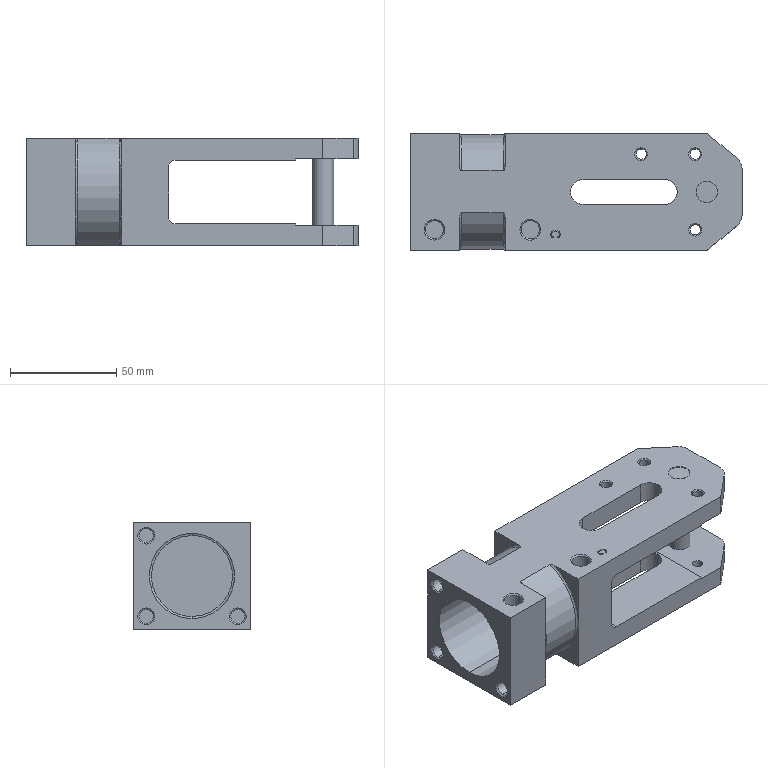Part | STEP file | 1 solid | 123 faces | box 156.007 x 55.626 x 50.292 mm | volume 208315 mm3 | cylinder 52 | plane 43 | cone 22 | spline 6 | commonest cylinder face diameters 4.917 x12 6.647 x6 10.104 x6 11.811 x6 8.566 x4 12.7 x4